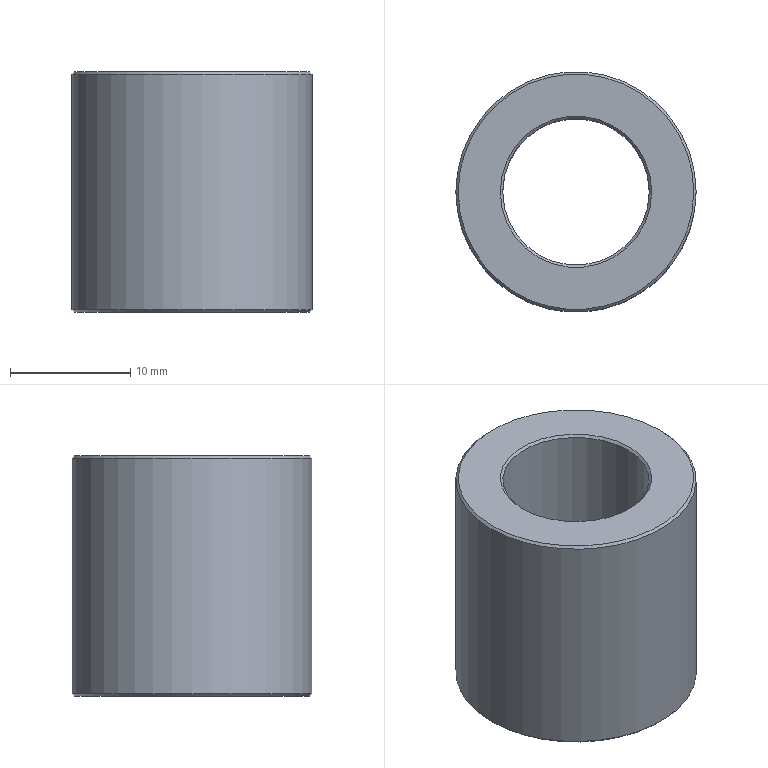Part | STEP file | PN_0015_default | 1 solid | 8 faces | box 20 x 20 x 20 mm | volume 3941 mm3 | cone 4 | plane 2 | cylinder 2 | commonest cylinder face diameters 12.2 x1 20 x1
STEP:
#1=CARTESIAN_POINT('',(0.,0.,0.));
#2=DIRECTION('',(0.,0.,1.));
#3=DIRECTION('',(1.,0.,0.));
#4=AXIS2_PLACEMENT_3D('',#1,#2,#3);
#5=CARTESIAN_POINT('',(6.3,0.,20.));
#6=VERTEX_POINT('',#5);
#7=CARTESIAN_POINT('',(0.,0.,20.));
#8=DIRECTION('',(0.,0.,-1.));
#9=DIRECTION('',(1.,0.,0.));
#10=AXIS2_PLACEMENT_3D('',#7,#8,#9);
#11=CIRCLE('',#10,6.3);
#12=CARTESIAN_POINT('',(0.,0.,20.));
#13=DIRECTION('',(0.,0.,1.));
#14=DIRECTION('',(1.,0.,0.));
#15=AXIS2_PLACEMENT_3D('',#12,#13,#14);
#16=PLANE('',#15);
#17=CARTESIAN_POINT('',(6.3,0.));
#18=CARTESIAN_POINT('',(6.3,-10.912));
#19=CARTESIAN_POINT('',(-3.15,-5.456));
#20=CARTESIAN_POINT('',(-12.6,0.));
#21=CARTESIAN_POINT('',(-3.15,5.456));
#22=CARTESIAN_POINT('',(6.3,10.912));
#23=CARTESIAN_POINT('',(6.3,0.));
#24=(BOUNDED_CURVE()B_SPLINE_CURVE(2,(#17,#18,#19,#20,#21,#22,#23),.UNSPECIFIED.,.T.,.F.)B_SPLINE_CURVE_WITH_KNOTS((1,2,2,2,2,1),(-2.094,0.,2.094,4.189,6.283,8.378),.UNSPECIFIED.)CURVE()GEOMETRIC_REPRESENTATION_ITEM()RATIONAL_B_SPLINE_CURVE((1.,0.5,1.,0.5,1.,0.5,1.))REPRESENTATION_ITEM(''));
#25=(GEOMETRIC_REPRESENTATION_CONTEXT(2)PARAMETRIC_REPRESENTATION_CONTEXT()REPRESENTATION_CONTEXT('',''));
#26=DEFINITIONAL_REPRESENTATION('',(#24),#25);
#27=PCURVE('',#16,#26);
#28=CARTESIAN_POINT('',(0.,0.,19.8));
#29=DIRECTION('',(0.,0.,1.));
#30=DIRECTION('',(1.,0.,0.));
#31=AXIS2_PLACEMENT_3D('',#28,#29,#30);
#32=CONICAL_SURFACE('',#31,6.1,0.7854);
#33=CARTESIAN_POINT('',(6.283,0.2));
#34=DIRECTION('',(-1.,0.));
#35=VECTOR('',#34,1.);
#36=LINE('',#33,#35);
#37=(GEOMETRIC_REPRESENTATION_CONTEXT(2)PARAMETRIC_REPRESENTATION_CONTEXT()REPRESENTATION_CONTEXT('',''));
#38=DEFINITIONAL_REPRESENTATION('',(#36),#37);
#39=PCURVE('',#32,#38);
#40=SURFACE_CURVE('',#11,(#27,#39),.PCURVE_S1.);
#41=EDGE_CURVE('',#6,#6,#40,.T.);
#42=ORIENTED_EDGE('',*,*,#41,.T.);
#43=EDGE_LOOP('',(#42));
#44=FACE_BOUND('',#43,.T.);
#45=CARTESIAN_POINT('',(9.8,0.,20.));
#46=VERTEX_POINT('',#45);
#47=CARTESIAN_POINT('',(0.,0.,20.));
#48=DIRECTION('',(0.,0.,1.));
#49=DIRECTION('',(1.,0.,0.));
#50=AXIS2_PLACEMENT_3D('',#47,#48,#49);
#51=CIRCLE('',#50,9.8);
#52=CARTESIAN_POINT('',(0.,0.));
#53=DIRECTION('',(1.,0.));
#54=AXIS2_PLACEMENT_2D('',#52,#53);
#55=CIRCLE('',#54,9.8);
#56=(GEOMETRIC_REPRESENTATION_CONTEXT(2)PARAMETRIC_REPRESENTATION_CONTEXT()REPRESENTATION_CONTEXT('',''));
#57=DEFINITIONAL_REPRESENTATION('',(#55),#56);
#58=PCURVE('',#16,#57);
#59=CARTESIAN_POINT('',(0.,0.,20.));
#60=DIRECTION('',(0.,0.,-1.));
#61=DIRECTION('',(-1.,0.,0.));
#62=AXIS2_PLACEMENT_3D('',#59,#60,#61);
#63=CONICAL_SURFACE('',#62,9.8,0.7854);
#64=CARTESIAN_POINT('',(9.425,0.));
#65=DIRECTION('',(-1.,0.));
#66=VECTOR('',#65,1.);
#67=LINE('',#64,#66);
#68=(GEOMETRIC_REPRESENTATION_CONTEXT(2)PARAMETRIC_REPRESENTATION_CONTEXT()REPRESENTATION_CONTEXT('',''));
#69=DEFINITIONAL_REPRESENTATION('',(#67),#68);
#70=PCURVE('',#63,#69);
#71=SURFACE_CURVE('',#51,(#58,#70),.PCURVE_S1.);
#72=EDGE_CURVE('',#46,#46,#71,.T.);
#73=ORIENTED_EDGE('',*,*,#72,.T.);
#74=EDGE_LOOP('',(#73));
#75=FACE_BOUND('',#74,.T.);
#76=ADVANCED_FACE('',(#44,#75),#16,.T.);
#77=CARTESIAN_POINT('',(6.3,0.,0.));
#78=VERTEX_POINT('',#77);
#79=CARTESIAN_POINT('',(0.,0.,0.));
#80=DIRECTION('',(0.,0.,1.));
#81=DIRECTION('',(1.,0.,0.));
#82=AXIS2_PLACEMENT_3D('',#79,#80,#81);
#83=CIRCLE('',#82,6.3);
#84=CARTESIAN_POINT('',(0.,0.,0.));
#85=DIRECTION('',(0.,0.,1.));
#86=DIRECTION('',(1.,0.,0.));
#87=AXIS2_PLACEMENT_3D('',#84,#85,#86);
#88=PLANE('',#87);
#89=CARTESIAN_POINT('',(0.,0.));
#90=DIRECTION('',(1.,0.));
#91=AXIS2_PLACEMENT_2D('',#89,#90);
#92=CIRCLE('',#91,6.3);
#93=(GEOMETRIC_REPRESENTATION_CONTEXT(2)PARAMETRIC_REPRESENTATION_CONTEXT()REPRESENTATION_CONTEXT('',''));
#94=DEFINITIONAL_REPRESENTATION('',(#92),#93);
#95=PCURVE('',#88,#94);
#96=CARTESIAN_POINT('',(0.,0.,0.));
#97=DIRECTION('',(0.,0.,-1.));
#98=DIRECTION('',(-1.,0.,0.));
#99=AXIS2_PLACEMENT_3D('',#96,#97,#98);
#100=CONICAL_SURFACE('',#99,6.3,0.7854);
#101=CARTESIAN_POINT('',(9.425,0.));
#102=DIRECTION('',(-1.,0.));
#103=VECTOR('',#102,1.);
#104=LINE('',#101,#103);
#105=(GEOMETRIC_REPRESENTATION_CONTEXT(2)PARAMETRIC_REPRESENTATION_CONTEXT()REPRESENTATION_CONTEXT('',''));
#106=DEFINITIONAL_REPRESENTATION('',(#104),#105);
#107=PCURVE('',#100,#106);
#108=SURFACE_CURVE('',#83,(#95,#107),.PCURVE_S1.);
#109=EDGE_CURVE('',#78,#78,#108,.T.);
#110=ORIENTED_EDGE('',*,*,#109,.T.);
#111=EDGE_LOOP('',(#110));
#112=FACE_BOUND('',#111,.T.);
#113=CARTESIAN_POINT('',(9.8,0.,0.));
#114=VERTEX_POINT('',#113);
#115=CARTESIAN_POINT('',(0.,0.,0.));
#116=DIRECTION('',(0.,0.,-1.));
#117=DIRECTION('',(1.,0.,0.));
#118=AXIS2_PLACEMENT_3D('',#115,#116,#117);
#119=CIRCLE('',#118,9.8);
#120=CARTESIAN_POINT('',(9.8,0.));
#121=CARTESIAN_POINT('',(9.8,-16.974));
#122=CARTESIAN_POINT('',(-4.9,-8.487));
#123=CARTESIAN_POINT('',(-19.6,0.));
#124=CARTESIAN_POINT('',(-4.9,8.487));
#125=CARTESIAN_POINT('',(9.8,16.974));
#126=CARTESIAN_POINT('',(9.8,0.));
#127=(BOUNDED_CURVE()B_SPLINE_CURVE(2,(#120,#121,#122,#123,#124,#125,#126),.UNSPECIFIED.,.T.,.F.)B_SPLINE_CURVE_WITH_KNOTS((1,2,2,2,2,1),(-2.094,0.,2.094,4.189,6.283,8.378),.UNSPECIFIED.)CURVE()GEOMETRIC_REPRESENTATION_ITEM()RATIONAL_B_SPLINE_CURVE((1.,0.5,1.,0.5,1.,0.5,1.))REPRESENTATION_ITEM(''));
#128=(GEOMETRIC_REPRESENTATION_CONTEXT(2)PARAMETRIC_REPRESENTATION_CONTEXT()REPRESENTATION_CONTEXT('',''));
#129=DEFINITIONAL_REPRESENTATION('',(#127),#128);
#130=PCURVE('',#88,#129);
#131=CARTESIAN_POINT('',(0.,0.,0.2));
#132=DIRECTION('',(0.,0.,1.));
#133=DIRECTION('',(1.,0.,0.));
#134=AXIS2_PLACEMENT_3D('',#131,#132,#133);
#135=CONICAL_SURFACE('',#134,10.,0.7854);
#136=CARTESIAN_POINT('',(6.283,-0.2));
#137=DIRECTION('',(-1.,0.));
#138=VECTOR('',#137,1.);
#139=LINE('',#136,#138);
#140=(GEOMETRIC_REPRESENTATION_CONTEXT(2)PARAMETRIC_REPRESENTATION_CONTEXT()REPRESENTATION_CONTEXT('',''));
#141=DEFINITIONAL_REPRESENTATION('',(#139),#140);
#142=PCURVE('',#135,#141);
#143=SURFACE_CURVE('',#119,(#130,#142),.PCURVE_S1.);
#144=EDGE_CURVE('',#114,#114,#143,.T.);
#145=ORIENTED_EDGE('',*,*,#144,.T.);
#146=EDGE_LOOP('',(#145));
#147=FACE_BOUND('',#146,.T.);
#148=ADVANCED_FACE('',(#112,#147),#88,.F.);
#149=CARTESIAN_POINT('',(10.,0.,0.2));
#150=VERTEX_POINT('',#149);
#151=CARTESIAN_POINT('',(0.,0.,0.2));
#152=DIRECTION('',(0.,0.,1.));
#153=DIRECTION('',(1.,0.,0.));
#154=AXIS2_PLACEMENT_3D('',#151,#152,#153);
#155=CIRCLE('',#154,10.);
#156=CARTESIAN_POINT('',(0.,0.,20.));
#157=DIRECTION('',(0.,0.,-1.));
#158=DIRECTION('',(-1.,0.,0.));
#159=AXIS2_PLACEMENT_3D('',#156,#157,#158);
#160=CYLINDRICAL_SURFACE('',#159,10.);
#161=CARTESIAN_POINT('',(9.425,19.8));
#162=DIRECTION('',(-1.,0.));
#163=VECTOR('',#162,1.);
#164=LINE('',#161,#163);
#165=(GEOMETRIC_REPRESENTATION_CONTEXT(2)PARAMETRIC_REPRESENTATION_CONTEXT()REPRESENTATION_CONTEXT('',''));
#166=DEFINITIONAL_REPRESENTATION('',(#164),#165);
#167=PCURVE('',#160,#166);
#168=CARTESIAN_POINT('',(0.,0.));
#169=DIRECTION('',(1.,0.));
#170=VECTOR('',#169,1.);
#171=LINE('',#168,#170);
#172=(GEOMETRIC_REPRESENTATION_CONTEXT(2)PARAMETRIC_REPRESENTATION_CONTEXT()REPRESENTATION_CONTEXT('',''));
#173=DEFINITIONAL_REPRESENTATION('',(#171),#172);
#174=PCURVE('',#135,#173);
#175=SURFACE_CURVE('',#155,(#167,#174),.PCURVE_S1.);
#176=EDGE_CURVE('',#150,#150,#175,.T.);
#177=ORIENTED_EDGE('',*,*,#176,.T.);
#178=CARTESIAN_POINT('',(10.,0.,19.8));
#179=VERTEX_POINT('',#178);
#180=CARTESIAN_POINT('',(10.,0.,19.8));
#181=CARTESIAN_POINT('',(10.,0.,0.2));
#182=B_SPLINE_CURVE_WITH_KNOTS('',1,(#180,#181),.UNSPECIFIED.,.F.,.F.,(2,2),(0.2,19.8),.PIECEWISE_BEZIER_KNOTS.);
#183=CARTESIAN_POINT('',(3.142,0.));
#184=DIRECTION('',(0.,1.));
#185=VECTOR('',#184,1.);
#186=LINE('',#183,#185);
#187=(GEOMETRIC_REPRESENTATION_CONTEXT(2)PARAMETRIC_REPRESENTATION_CONTEXT()REPRESENTATION_CONTEXT('',''));
#188=DEFINITIONAL_REPRESENTATION('',(#186),#187);
#189=PCURVE('',#160,#188);
#190=CARTESIAN_POINT('',(9.425,0.));
#191=DIRECTION('',(0.,1.));
#192=VECTOR('',#191,1.);
#193=LINE('',#190,#192);
#194=(GEOMETRIC_REPRESENTATION_CONTEXT(2)PARAMETRIC_REPRESENTATION_CONTEXT()REPRESENTATION_CONTEXT('',''));
#195=DEFINITIONAL_REPRESENTATION('',(#193),#194);
#196=PCURVE('',#160,#195);
#197=SEAM_CURVE('',#182,(#189,#196),.PCURVE_S1.);
#198=EDGE_CURVE('',#179,#150,#197,.T.);
#199=ORIENTED_EDGE('',*,*,#198,.F.);
#200=CARTESIAN_POINT('',(0.,0.,19.8));
#201=DIRECTION('',(0.,0.,-1.));
#202=DIRECTION('',(1.,0.,0.));
#203=AXIS2_PLACEMENT_3D('',#200,#201,#202);
#204=CIRCLE('',#203,10.);
#205=CARTESIAN_POINT('',(3.142,0.2));
#206=DIRECTION('',(1.,0.));
#207=VECTOR('',#206,1.);
#208=LINE('',#205,#207);
#209=(GEOMETRIC_REPRESENTATION_CONTEXT(2)PARAMETRIC_REPRESENTATION_CONTEXT()REPRESENTATION_CONTEXT('',''));
#210=DEFINITIONAL_REPRESENTATION('',(#208),#209);
#211=PCURVE('',#160,#210);
#212=CARTESIAN_POINT('',(3.142,0.2));
#213=DIRECTION('',(1.,0.));
#214=VECTOR('',#213,1.);
#215=LINE('',#212,#214);
#216=(GEOMETRIC_REPRESENTATION_CONTEXT(2)PARAMETRIC_REPRESENTATION_CONTEXT()REPRESENTATION_CONTEXT('',''));
#217=DEFINITIONAL_REPRESENTATION('',(#215),#216);
#218=PCURVE('',#63,#217);
#219=SURFACE_CURVE('',#204,(#211,#218),.PCURVE_S1.);
#220=EDGE_CURVE('',#179,#179,#219,.T.);
#221=ORIENTED_EDGE('',*,*,#220,.T.);
#222=ORIENTED_EDGE('',*,*,#198,.T.);
#223=EDGE_LOOP('',(#177,#199,#221,#222));
#224=FACE_BOUND('',#223,.T.);
#225=ADVANCED_FACE('',(#224),#160,.T.);
#226=CARTESIAN_POINT('',(6.1,0.,0.2));
#227=VERTEX_POINT('',#226);
#228=CARTESIAN_POINT('',(0.,0.,0.2));
#229=DIRECTION('',(0.,0.,-1.));
#230=DIRECTION('',(1.,0.,0.));
#231=AXIS2_PLACEMENT_3D('',#228,#229,#230);
#232=CIRCLE('',#231,6.1);
#233=CARTESIAN_POINT('',(0.,0.,20.));
#234=DIRECTION('',(0.,0.,-1.));
#235=DIRECTION('',(-1.,0.,0.));
#236=AXIS2_PLACEMENT_3D('',#233,#234,#235);
#237=CYLINDRICAL_SURFACE('',#236,6.1);
#238=CARTESIAN_POINT('',(3.142,19.8));
#239=DIRECTION('',(1.,0.));
#240=VECTOR('',#239,1.);
#241=LINE('',#238,#240);
#242=(GEOMETRIC_REPRESENTATION_CONTEXT(2)PARAMETRIC_REPRESENTATION_CONTEXT()REPRESENTATION_CONTEXT('',''));
#243=DEFINITIONAL_REPRESENTATION('',(#241),#242);
#244=PCURVE('',#237,#243);
#245=CARTESIAN_POINT('',(3.142,-0.2));
#246=DIRECTION('',(1.,0.));
#247=VECTOR('',#246,1.);
#248=LINE('',#245,#247);
#249=(GEOMETRIC_REPRESENTATION_CONTEXT(2)PARAMETRIC_REPRESENTATION_CONTEXT()REPRESENTATION_CONTEXT('',''));
#250=DEFINITIONAL_REPRESENTATION('',(#248),#249);
#251=PCURVE('',#100,#250);
#252=SURFACE_CURVE('',#232,(#244,#251),.PCURVE_S1.);
#253=EDGE_CURVE('',#227,#227,#252,.T.);
#254=ORIENTED_EDGE('',*,*,#253,.F.);
#255=CARTESIAN_POINT('',(6.1,0.,19.8));
#256=VERTEX_POINT('',#255);
#257=CARTESIAN_POINT('',(6.1,0.,19.8));
#258=CARTESIAN_POINT('',(6.1,0.,0.2));
#259=B_SPLINE_CURVE_WITH_KNOTS('',1,(#257,#258),.UNSPECIFIED.,.F.,.F.,(2,2),(0.2,19.8),.PIECEWISE_BEZIER_KNOTS.);
#260=CARTESIAN_POINT('',(3.142,0.));
#261=DIRECTION('',(0.,1.));
#262=VECTOR('',#261,1.);
#263=LINE('',#260,#262);
#264=(GEOMETRIC_REPRESENTATION_CONTEXT(2)PARAMETRIC_REPRESENTATION_CONTEXT()REPRESENTATION_CONTEXT('',''));
#265=DEFINITIONAL_REPRESENTATION('',(#263),#264);
#266=PCURVE('',#237,#265);
#267=CARTESIAN_POINT('',(9.425,0.));
#268=DIRECTION('',(0.,1.));
#269=VECTOR('',#268,1.);
#270=LINE('',#267,#269);
#271=(GEOMETRIC_REPRESENTATION_CONTEXT(2)PARAMETRIC_REPRESENTATION_CONTEXT()REPRESENTATION_CONTEXT('',''));
#272=DEFINITIONAL_REPRESENTATION('',(#270),#271);
#273=PCURVE('',#237,#272);
#274=SEAM_CURVE('',#259,(#266,#273),.PCURVE_S1.);
#275=EDGE_CURVE('',#256,#227,#274,.T.);
#276=ORIENTED_EDGE('',*,*,#275,.F.);
#277=CARTESIAN_POINT('',(0.,0.,19.8));
#278=DIRECTION('',(0.,0.,1.));
#279=DIRECTION('',(1.,0.,0.));
#280=AXIS2_PLACEMENT_3D('',#277,#278,#279);
#281=CIRCLE('',#280,6.1);
#282=CARTESIAN_POINT('',(9.425,0.2));
#283=DIRECTION('',(-1.,0.));
#284=VECTOR('',#283,1.);
#285=LINE('',#282,#284);
#286=(GEOMETRIC_REPRESENTATION_CONTEXT(2)PARAMETRIC_REPRESENTATION_CONTEXT()REPRESENTATION_CONTEXT('',''));
#287=DEFINITIONAL_REPRESENTATION('',(#285),#286);
#288=PCURVE('',#237,#287);
#289=CARTESIAN_POINT('',(0.,0.));
#290=DIRECTION('',(1.,0.));
#291=VECTOR('',#290,1.);
#292=LINE('',#289,#291);
#293=(GEOMETRIC_REPRESENTATION_CONTEXT(2)PARAMETRIC_REPRESENTATION_CONTEXT()REPRESENTATION_CONTEXT('',''));
#294=DEFINITIONAL_REPRESENTATION('',(#292),#293);
#295=PCURVE('',#32,#294);
#296=SURFACE_CURVE('',#281,(#288,#295),.PCURVE_S1.);
#297=EDGE_CURVE('',#256,#256,#296,.T.);
#298=ORIENTED_EDGE('',*,*,#297,.F.);
#299=ORIENTED_EDGE('',*,*,#275,.T.);
#300=EDGE_LOOP('',(#254,#276,#298,#299));
#301=FACE_BOUND('',#300,.F.);
#302=ADVANCED_FACE('',(#301),#237,.F.);
#303=ORIENTED_EDGE('',*,*,#253,.T.);
#304=CARTESIAN_POINT('',(6.1,0.,0.2));
#305=CARTESIAN_POINT('',(6.3,0.,0.));
#306=B_SPLINE_CURVE_WITH_KNOTS('',1,(#304,#305),.UNSPECIFIED.,.F.,.F.,(2,2),(-0.2828,0.),.PIECEWISE_BEZIER_KNOTS.);
#307=CARTESIAN_POINT('',(9.425,0.));
#308=DIRECTION('',(0.,1.));
#309=VECTOR('',#308,1.);
#310=LINE('',#307,#309);
#311=(GEOMETRIC_REPRESENTATION_CONTEXT(2)PARAMETRIC_REPRESENTATION_CONTEXT()REPRESENTATION_CONTEXT('',''));
#312=DEFINITIONAL_REPRESENTATION('',(#310),#311);
#313=PCURVE('',#100,#312);
#314=CARTESIAN_POINT('',(3.142,0.));
#315=DIRECTION('',(0.,1.));
#316=VECTOR('',#315,1.);
#317=LINE('',#314,#316);
#318=(GEOMETRIC_REPRESENTATION_CONTEXT(2)PARAMETRIC_REPRESENTATION_CONTEXT()REPRESENTATION_CONTEXT('',''));
#319=DEFINITIONAL_REPRESENTATION('',(#317),#318);
#320=PCURVE('',#100,#319);
#321=SEAM_CURVE('',#306,(#313,#320),.PCURVE_S1.);
#322=EDGE_CURVE('',#227,#78,#321,.T.);
#323=ORIENTED_EDGE('',*,*,#322,.T.);
#324=ORIENTED_EDGE('',*,*,#109,.T.);
#325=ORIENTED_EDGE('',*,*,#322,.F.);
#326=EDGE_LOOP('',(#303,#323,#324,#325));
#327=FACE_BOUND('',#326,.F.);
#328=ADVANCED_FACE('',(#327),#100,.F.);
#329=ORIENTED_EDGE('',*,*,#144,.F.);
#330=CARTESIAN_POINT('',(9.8,0.,0.));
#331=CARTESIAN_POINT('',(10.,0.,0.2));
#332=B_SPLINE_CURVE_WITH_KNOTS('',1,(#330,#331),.UNSPECIFIED.,.F.,.F.,(2,2),(-0.2828,0.),.PIECEWISE_BEZIER_KNOTS.);
#333=CARTESIAN_POINT('',(6.283,0.));
#334=DIRECTION('',(0.,1.));
#335=VECTOR('',#334,1.);
#336=LINE('',#333,#335);
#337=(GEOMETRIC_REPRESENTATION_CONTEXT(2)PARAMETRIC_REPRESENTATION_CONTEXT()REPRESENTATION_CONTEXT('',''));
#338=DEFINITIONAL_REPRESENTATION('',(#336),#337);
#339=PCURVE('',#135,#338);
#340=CARTESIAN_POINT('',(0.,0.));
#341=DIRECTION('',(0.,1.));
#342=VECTOR('',#341,1.);
#343=LINE('',#340,#342);
#344=(GEOMETRIC_REPRESENTATION_CONTEXT(2)PARAMETRIC_REPRESENTATION_CONTEXT()REPRESENTATION_CONTEXT('',''));
#345=DEFINITIONAL_REPRESENTATION('',(#343),#344);
#346=PCURVE('',#135,#345);
#347=SEAM_CURVE('',#332,(#339,#346),.PCURVE_S1.);
#348=EDGE_CURVE('',#114,#150,#347,.T.);
#349=ORIENTED_EDGE('',*,*,#348,.T.);
#350=ORIENTED_EDGE('',*,*,#176,.F.);
#351=ORIENTED_EDGE('',*,*,#348,.F.);
#352=EDGE_LOOP('',(#329,#349,#350,#351));
#353=FACE_BOUND('',#352,.T.);
#354=ADVANCED_FACE('',(#353),#135,.T.);
#355=ORIENTED_EDGE('',*,*,#41,.T.);
#356=CARTESIAN_POINT('',(6.1,0.,19.8));
#357=CARTESIAN_POINT('',(6.3,0.,20.));
#358=B_SPLINE_CURVE_WITH_KNOTS('',1,(#356,#357),.UNSPECIFIED.,.F.,.F.,(2,2),(0.,0.2828),.PIECEWISE_BEZIER_KNOTS.);
#359=CARTESIAN_POINT('',(0.,0.));
#360=DIRECTION('',(0.,1.));
#361=VECTOR('',#360,1.);
#362=LINE('',#359,#361);
#363=(GEOMETRIC_REPRESENTATION_CONTEXT(2)PARAMETRIC_REPRESENTATION_CONTEXT()REPRESENTATION_CONTEXT('',''));
#364=DEFINITIONAL_REPRESENTATION('',(#362),#363);
#365=PCURVE('',#32,#364);
#366=CARTESIAN_POINT('',(6.283,0.));
#367=DIRECTION('',(0.,1.));
#368=VECTOR('',#367,1.);
#369=LINE('',#366,#368);
#370=(GEOMETRIC_REPRESENTATION_CONTEXT(2)PARAMETRIC_REPRESENTATION_CONTEXT()REPRESENTATION_CONTEXT('',''));
#371=DEFINITIONAL_REPRESENTATION('',(#369),#370);
#372=PCURVE('',#32,#371);
#373=SEAM_CURVE('',#358,(#365,#372),.PCURVE_S1.);
#374=EDGE_CURVE('',#256,#6,#373,.T.);
#375=ORIENTED_EDGE('',*,*,#374,.F.);
#376=ORIENTED_EDGE('',*,*,#297,.T.);
#377=ORIENTED_EDGE('',*,*,#374,.T.);
#378=EDGE_LOOP('',(#355,#375,#376,#377));
#379=FACE_BOUND('',#378,.F.);
#380=ADVANCED_FACE('',(#379),#32,.F.);
#381=ORIENTED_EDGE('',*,*,#220,.F.);
#382=CARTESIAN_POINT('',(9.8,0.,20.));
#383=CARTESIAN_POINT('',(10.,0.,19.8));
#384=B_SPLINE_CURVE_WITH_KNOTS('',1,(#382,#383),.UNSPECIFIED.,.F.,.F.,(2,2),(0.,0.2828),.PIECEWISE_BEZIER_KNOTS.);
#385=CARTESIAN_POINT('',(3.142,0.));
#386=DIRECTION('',(0.,1.));
#387=VECTOR('',#386,1.);
#388=LINE('',#385,#387);
#389=(GEOMETRIC_REPRESENTATION_CONTEXT(2)PARAMETRIC_REPRESENTATION_CONTEXT()REPRESENTATION_CONTEXT('',''));
#390=DEFINITIONAL_REPRESENTATION('',(#388),#389);
#391=PCURVE('',#63,#390);
#392=CARTESIAN_POINT('',(9.425,0.));
#393=DIRECTION('',(0.,1.));
#394=VECTOR('',#393,1.);
#395=LINE('',#392,#394);
#396=(GEOMETRIC_REPRESENTATION_CONTEXT(2)PARAMETRIC_REPRESENTATION_CONTEXT()REPRESENTATION_CONTEXT('',''));
#397=DEFINITIONAL_REPRESENTATION('',(#395),#396);
#398=PCURVE('',#63,#397);
#399=SEAM_CURVE('',#384,(#391,#398),.PCURVE_S1.);
#400=EDGE_CURVE('',#46,#179,#399,.T.);
#401=ORIENTED_EDGE('',*,*,#400,.F.);
#402=ORIENTED_EDGE('',*,*,#72,.F.);
#403=ORIENTED_EDGE('',*,*,#400,.T.);
#404=EDGE_LOOP('',(#381,#401,#402,#403));
#405=FACE_BOUND('',#404,.T.);
#406=ADVANCED_FACE('',(#405),#63,.T.);
#407=CLOSED_SHELL('',(#76,#148,#225,#302,#328,#354,#380,#406));
#408=MANIFOLD_SOLID_BREP('',#407);
#409=(LENGTH_UNIT()NAMED_UNIT(*)SI_UNIT(.MILLI.,.METRE.));
#410=UNCERTAINTY_MEASURE_WITH_UNIT(LENGTH_MEASURE(0.00001),#409,'','');
#411=(NAMED_UNIT(*)PLANE_ANGLE_UNIT()SI_UNIT($,.RADIAN.));
#412=(NAMED_UNIT(*)SI_UNIT($,.STERADIAN.)SOLID_ANGLE_UNIT());
#413=(GEOMETRIC_REPRESENTATION_CONTEXT(3)GLOBAL_UNCERTAINTY_ASSIGNED_CONTEXT((#410))GLOBAL_UNIT_ASSIGNED_CONTEXT((#409,#411,#412))REPRESENTATION_CONTEXT('',''));
#414=ADVANCED_BREP_SHAPE_REPRESENTATION('',(#4,#408),#413);